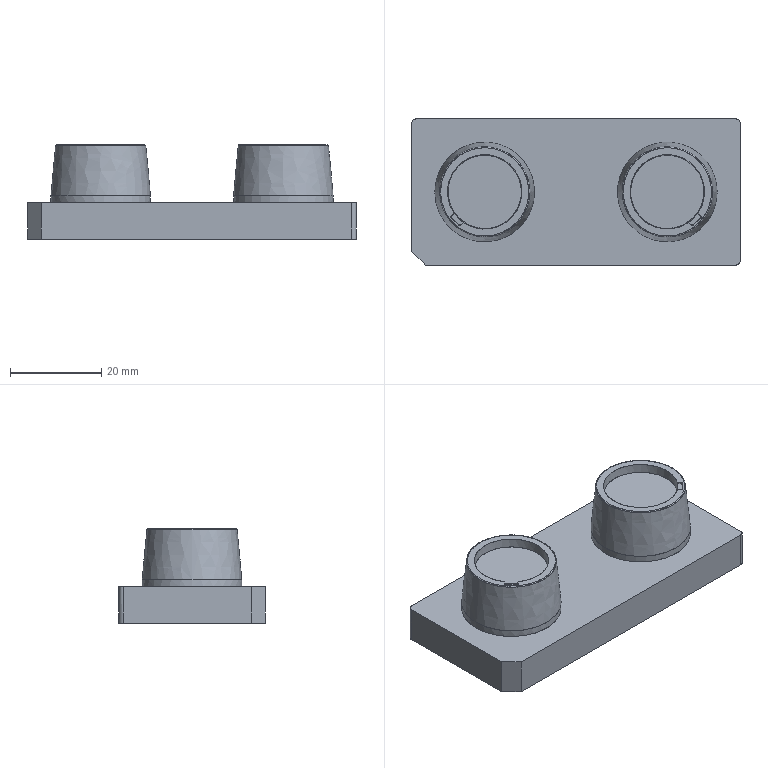CAM job | PowerMill | 3-axis milling, other | part box 72 x 32 x 20.655 mm
Tools:
number,name,type,diameter,tip_radius,length,cutting_length,overhang,flutes,holder,toolpaths_using
1,D10C,end_mill,10.0,0.0,60.0,,30.0,1,D42L35,1
8,D1_1,end_mill,1.0,0.0,3.0,,1.0,1,D42L35,2
1,D10C_1_1_1,end_mill,10.0,0.0,60.0,,21.12,1,D42L35,3
2,D4C_1_1,end_mill,4.0,0.0,30.0,,12.84,1,D42L35,1
3,D10_1_1_1,end_mill,10.0,0.0,60.0,,20.8,1,D42L35,4
5,B4R0.5_1_1,tip_radiused,4.0,0.5,30.0,,12.8,1,D42L35,2
13,Text_D4_1_1,taper_spherical,4.0,0.3,60.0,,12.92,1,D42L35,1
Operations:
program,toolpath,strategy,tool,tool_number,tool_diameter,tip_radius,flutes,spindle_rpm,feed_cut,surface_speed_m_min_computed,feed_per_tooth_computed,tolerance,thickness,stepover,stepdown,cut_length,cut_time_min,total_time_min,workplane
25-B01-1-F,精公开粗01-扫面平行-D10C,raster_area_clear,D10C_1_1_1,1,10.0,0.0,1.0,8000.0,10000.0,251.33,1.25,0.03,0.28,6.0,1.0,658.04,0.066,0.0737,
25-B01-1-F,精公开粗01-外形偏置-D10C,offset_area_clear,D10C_1_1_1,1,10.0,0.0,1.0,8000.0,10000.0,251.33,1.25,0.03,0.28,6.0,1.0,15663.438,1.566,1.718,
25-B01-1-F,精公开粗01-基准台等高-D10C,constantz,D10C_1_1_1,1,10.0,0.0,1.0,8000.0,10000.0,251.33,1.25,0.03,0.07,5.0,0.4,5209.022,0.521,0.533,
25-B01-1-F,精公再粗02-外形偏置-D4C,offset_area_clear,D4C_1_1,2,4.0,0.0,1.0,18000.0,6000.0,226.19,0.3333,0.03,0.0,2.0,1.0,12619.625,2.103,2.286,
25-B01-1-F,精公基准台01-平坦面平行-D10,raster_area_clear,D10_1_1_1,3,10.0,0.0,1.0,8500.0,600.0,267.04,0.0706,0.005,0.38,5.0,1.0,363.666,0.606,0.6424,
25-B01-1-F,精公基准台01-基准面偏置-D10,offset_area_clear,D10_1_1_1,3,10.0,0.0,1.0,8500.0,600.0,267.04,0.0706,0.005,0.38,5.0,1.0,365.033,0.608,0.6496,
25-B01-1-F,精公基准台01-外形侧光-D10,profile_area_clear,D10_1_1_1,3,10.0,0.0,1.0,8500.0,600.0,267.04,0.0706,0.005,-0.07,0.08,1.0,398.798,0.665,0.7074,
25-B01-1-F,精公基准台01-基准台侧光-D10,profile_area_clear,D10_1_1_1,3,10.0,0.0,1.0,8500.0,600.0,267.04,0.0706,0.005,0.0,0.08,1.0,473.233,0.789,0.8554,
25-B01-1-F,精公精光01-等高-B4R0.5,constantz,B4R0.5_1_1,5,4.0,0.5,1.0,18000.0,2000.0,226.19,0.1111,0.005,-0.075,5.0,0.02,52990.323,26.495,27.718,
25-B01-1-F,精公精光01-平坦面偏置-B4R0.5,offset_area_clear,B4R0.5_1_1,5,4.0,0.5,1.0,18000.0,600.0,226.19,0.0333,0.005,0.375,2.0,1.0,385.959,0.643,0.761,
25-B01-1-F,精公精光02-等高-D1,constantz,D1_1,8,1.0,0.0,1.0,20000.0,1000.0,62.83,0.05,0.005,-0.075,5.0,0.02,151.427,0.151,0.1865,
25-B01-1-F,精公精光02-平坦面偏置-D1,offset_area_clear,D1_1,8,1.0,0.0,1.0,20000.0,600.0,62.83,0.03,0.005,0.375,0.5,1.0,5.378,0.009,0.0584,
25-B01-1-F,精公刻字01-刻字-Text_D4,pattern,Text_D4_1_1,13,4.0,0.3,1.0,15000.0,1000.0,188.5,0.0667,0.005,0.0,5.0,1.0,56.451,0.057,0.0756,
,精公开粗01-外形偏置-D10C_Reference,offset_area_clear,D10C,1,10.0,0.0,1.0,8000.0,10000.0,251.33,1.25,0.03,0.28,6.0,1.0,30501.868,3.05,3.207,